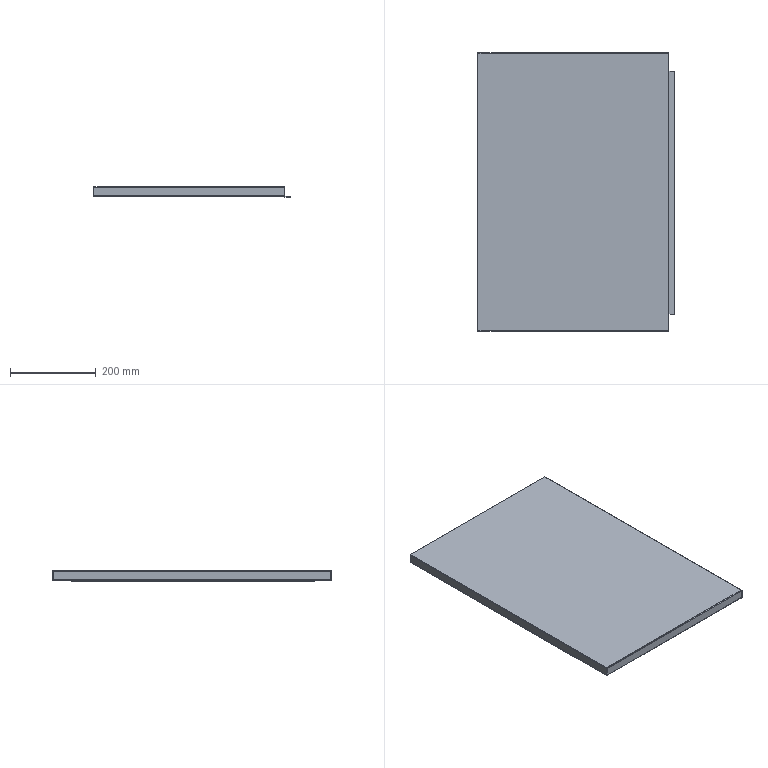Part | SolidWorks | features EdgeFlange 4, FlatPattern 1, ICE 1, SMBaseFlange 1, SheetMetal 1 | 1 solid | 84 faces | box 460.5 x 650 x 23.5 mm | volume 531757 mm3 | plane 56 | cylinder 20 | spline 8 | commonest cylinder face diameters 0.2 x8 3.2 x8 4 x4